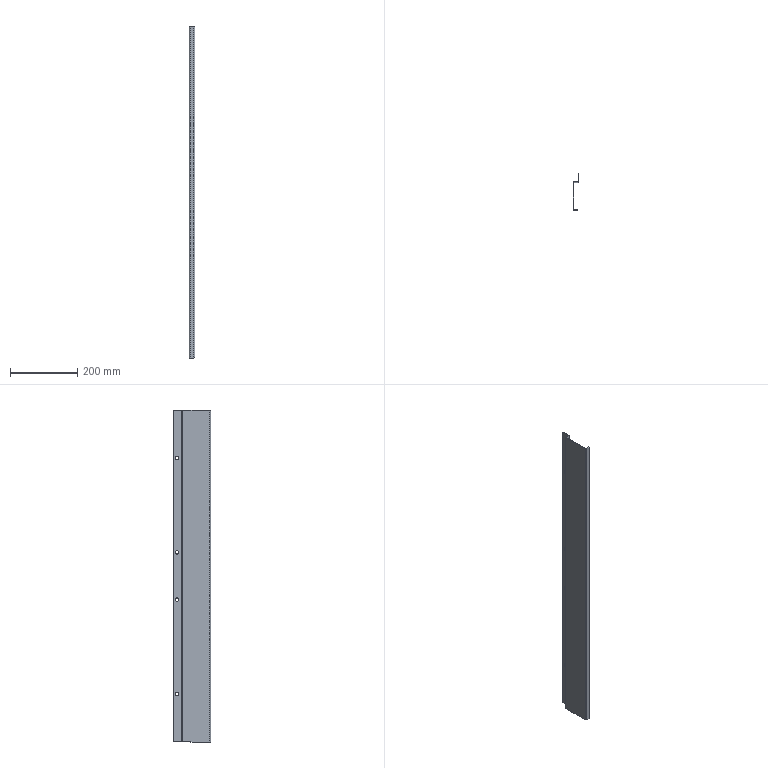Part | STEP file | 750038331 | 1 solid | 30 faces | box 16.25 x 110 x 985 mm | volume 264288 mm3 | plane 16 | cylinder 14 | commonest cylinder face diameters 10.5 x8 0.5 x3 4.5 x3
STEP:
#1=CARTESIAN_POINT('',(16.25,100.,355.25));
#2=VERTEX_POINT('',#1);
#3=CARTESIAN_POINT('',(16.25,100.,344.75));
#4=VERTEX_POINT('',#3);
#5=CARTESIAN_POINT('',(16.25,100.,350.));
#6=DIRECTION('',(1.,0.,0.));
#7=DIRECTION('',(0.,0.,1.));
#8=AXIS2_PLACEMENT_3D('',#5,#6,#7);
#9=CIRCLE('',#8,5.25);
#10=EDGE_CURVE('',#2,#4,#9,.T.);
#11=ORIENTED_EDGE('',*,*,#10,.T.);
#12=CARTESIAN_POINT('',(14.25,100.,344.75));
#13=VERTEX_POINT('',#12);
#14=CARTESIAN_POINT('',(1005.506,100.,344.75));
#15=DIRECTION('',(-1.,0.,0.));
#16=VECTOR('',#15,1000.);
#17=LINE('',#14,#16);
#18=EDGE_CURVE('',#4,#13,#17,.T.);
#19=ORIENTED_EDGE('',*,*,#18,.T.);
#20=CARTESIAN_POINT('',(14.25,100.,355.25));
#21=VERTEX_POINT('',#20);
#22=CARTESIAN_POINT('',(14.25,100.,350.));
#23=DIRECTION('',(1.,0.,0.));
#24=DIRECTION('',(0.,0.,1.));
#25=AXIS2_PLACEMENT_3D('',#22,#23,#24);
#26=CIRCLE('',#25,5.25);
#27=EDGE_CURVE('',#21,#13,#26,.T.);
#28=ORIENTED_EDGE('',*,*,#27,.F.);
#29=CARTESIAN_POINT('',(1005.506,100.,355.25));
#30=DIRECTION('',(-1.,0.,0.));
#31=VECTOR('',#30,1000.);
#32=LINE('',#29,#31);
#33=EDGE_CURVE('',#2,#21,#32,.T.);
#34=ORIENTED_EDGE('',*,*,#33,.F.);
#35=EDGE_LOOP('',(#11,#19,#28,#34));
#36=FACE_OUTER_BOUND('',#35,.T.);
#37=CARTESIAN_POINT('',(1005.506,100.,350.));
#38=DIRECTION('',(-1.,0.,0.));
#39=DIRECTION('',(0.,0.,1.));
#40=AXIS2_PLACEMENT_3D('',#37,#38,#39);
#41=CYLINDRICAL_SURFACE('',#40,5.25);
#42=ADVANCED_FACE('',(#36),#41,.F.);
#43=CARTESIAN_POINT('',(16.25,100.,75.25));
#44=VERTEX_POINT('',#43);
#45=CARTESIAN_POINT('',(16.25,100.,64.75));
#46=VERTEX_POINT('',#45);
#47=CARTESIAN_POINT('',(16.25,100.,70.));
#48=DIRECTION('',(1.,0.,0.));
#49=DIRECTION('',(0.,0.,1.));
#50=AXIS2_PLACEMENT_3D('',#47,#48,#49);
#51=CIRCLE('',#50,5.25);
#52=EDGE_CURVE('',#44,#46,#51,.T.);
#53=ORIENTED_EDGE('',*,*,#52,.T.);
#54=CARTESIAN_POINT('',(14.25,100.,64.75));
#55=VERTEX_POINT('',#54);
#56=CARTESIAN_POINT('',(1005.506,100.,64.75));
#57=DIRECTION('',(-1.,0.,0.));
#58=VECTOR('',#57,1000.);
#59=LINE('',#56,#58);
#60=EDGE_CURVE('',#46,#55,#59,.T.);
#61=ORIENTED_EDGE('',*,*,#60,.T.);
#62=CARTESIAN_POINT('',(14.25,100.,75.25));
#63=VERTEX_POINT('',#62);
#64=CARTESIAN_POINT('',(14.25,100.,70.));
#65=DIRECTION('',(1.,0.,0.));
#66=DIRECTION('',(0.,0.,1.));
#67=AXIS2_PLACEMENT_3D('',#64,#65,#66);
#68=CIRCLE('',#67,5.25);
#69=EDGE_CURVE('',#63,#55,#68,.T.);
#70=ORIENTED_EDGE('',*,*,#69,.F.);
#71=CARTESIAN_POINT('',(1005.506,100.,75.25));
#72=DIRECTION('',(-1.,0.,0.));
#73=VECTOR('',#72,1000.);
#74=LINE('',#71,#73);
#75=EDGE_CURVE('',#44,#63,#74,.T.);
#76=ORIENTED_EDGE('',*,*,#75,.F.);
#77=EDGE_LOOP('',(#53,#61,#70,#76));
#78=FACE_OUTER_BOUND('',#77,.T.);
#79=CARTESIAN_POINT('',(1005.506,100.,70.));
#80=DIRECTION('',(-1.,0.,0.));
#81=DIRECTION('',(0.,0.,1.));
#82=AXIS2_PLACEMENT_3D('',#79,#80,#81);
#83=CYLINDRICAL_SURFACE('',#82,5.25);
#84=ADVANCED_FACE('',(#78),#83,.F.);
#85=CARTESIAN_POINT('',(16.25,100.,-344.75));
#86=VERTEX_POINT('',#85);
#87=CARTESIAN_POINT('',(16.25,100.,-355.25));
#88=VERTEX_POINT('',#87);
#89=CARTESIAN_POINT('',(16.25,100.,-350.));
#90=DIRECTION('',(1.,0.,0.));
#91=DIRECTION('',(0.,0.,1.));
#92=AXIS2_PLACEMENT_3D('',#89,#90,#91);
#93=CIRCLE('',#92,5.25);
#94=EDGE_CURVE('',#86,#88,#93,.T.);
#95=ORIENTED_EDGE('',*,*,#94,.T.);
#96=CARTESIAN_POINT('',(14.25,100.,-355.25));
#97=VERTEX_POINT('',#96);
#98=CARTESIAN_POINT('',(1005.506,100.,-355.25));
#99=DIRECTION('',(-1.,0.,0.));
#100=VECTOR('',#99,1000.);
#101=LINE('',#98,#100);
#102=EDGE_CURVE('',#88,#97,#101,.T.);
#103=ORIENTED_EDGE('',*,*,#102,.T.);
#104=CARTESIAN_POINT('',(14.25,100.,-344.75));
#105=VERTEX_POINT('',#104);
#106=CARTESIAN_POINT('',(14.25,100.,-350.));
#107=DIRECTION('',(1.,0.,0.));
#108=DIRECTION('',(0.,0.,1.));
#109=AXIS2_PLACEMENT_3D('',#106,#107,#108);
#110=CIRCLE('',#109,5.25);
#111=EDGE_CURVE('',#105,#97,#110,.T.);
#112=ORIENTED_EDGE('',*,*,#111,.F.);
#113=CARTESIAN_POINT('',(1005.506,100.,-344.75));
#114=DIRECTION('',(-1.,0.,0.));
#115=VECTOR('',#114,1000.);
#116=LINE('',#113,#115);
#117=EDGE_CURVE('',#86,#105,#116,.T.);
#118=ORIENTED_EDGE('',*,*,#117,.F.);
#119=EDGE_LOOP('',(#95,#103,#112,#118));
#120=FACE_OUTER_BOUND('',#119,.T.);
#121=CARTESIAN_POINT('',(1005.506,100.,-350.));
#122=DIRECTION('',(-1.,0.,0.));
#123=DIRECTION('',(0.,0.,1.));
#124=AXIS2_PLACEMENT_3D('',#121,#122,#123);
#125=CYLINDRICAL_SURFACE('',#124,5.25);
#126=ADVANCED_FACE('',(#120),#125,.F.);
#127=CARTESIAN_POINT('',(16.25,100.,-64.75));
#128=VERTEX_POINT('',#127);
#129=CARTESIAN_POINT('',(16.25,100.,-75.25));
#130=VERTEX_POINT('',#129);
#131=CARTESIAN_POINT('',(16.25,100.,-70.));
#132=DIRECTION('',(1.,0.,0.));
#133=DIRECTION('',(0.,0.,1.));
#134=AXIS2_PLACEMENT_3D('',#131,#132,#133);
#135=CIRCLE('',#134,5.25);
#136=EDGE_CURVE('',#128,#130,#135,.T.);
#137=ORIENTED_EDGE('',*,*,#136,.T.);
#138=CARTESIAN_POINT('',(14.25,100.,-75.25));
#139=VERTEX_POINT('',#138);
#140=CARTESIAN_POINT('',(1005.506,100.,-75.25));
#141=DIRECTION('',(-1.,0.,0.));
#142=VECTOR('',#141,1000.);
#143=LINE('',#140,#142);
#144=EDGE_CURVE('',#130,#139,#143,.T.);
#145=ORIENTED_EDGE('',*,*,#144,.T.);
#146=CARTESIAN_POINT('',(14.25,100.,-64.75));
#147=VERTEX_POINT('',#146);
#148=CARTESIAN_POINT('',(14.25,100.,-70.));
#149=DIRECTION('',(1.,0.,0.));
#150=DIRECTION('',(0.,0.,1.));
#151=AXIS2_PLACEMENT_3D('',#148,#149,#150);
#152=CIRCLE('',#151,5.25);
#153=EDGE_CURVE('',#147,#139,#152,.T.);
#154=ORIENTED_EDGE('',*,*,#153,.F.);
#155=CARTESIAN_POINT('',(1005.506,100.,-64.75));
#156=DIRECTION('',(-1.,0.,0.));
#157=VECTOR('',#156,1000.);
#158=LINE('',#155,#157);
#159=EDGE_CURVE('',#128,#147,#158,.T.);
#160=ORIENTED_EDGE('',*,*,#159,.F.);
#161=EDGE_LOOP('',(#137,#145,#154,#160));
#162=FACE_OUTER_BOUND('',#161,.T.);
#163=CARTESIAN_POINT('',(1005.506,100.,-70.));
#164=DIRECTION('',(-1.,0.,0.));
#165=DIRECTION('',(0.,0.,1.));
#166=AXIS2_PLACEMENT_3D('',#163,#164,#165);
#167=CYLINDRICAL_SURFACE('',#166,5.25);
#168=ADVANCED_FACE('',(#162),#167,.F.);
#169=CARTESIAN_POINT('',(0.,83.75,491.5));
#170=VERTEX_POINT('',#169);
#171=CARTESIAN_POINT('',(0.,83.75,-491.5));
#172=VERTEX_POINT('',#171);
#173=CARTESIAN_POINT('',(0.,83.75,492.5));
#174=DIRECTION('',(0.,0.,-1.));
#175=VECTOR('',#174,1000.);
#176=LINE('',#173,#175);
#177=EDGE_CURVE('',#170,#172,#176,.T.);
#178=ORIENTED_EDGE('',*,*,#177,.T.);
#179=CARTESIAN_POINT('',(0.,58.,-491.5));
#180=VERTEX_POINT('',#179);
#181=CARTESIAN_POINT('',(0.,0.,-491.5));
#182=DIRECTION('',(0.,-1.,0.));
#183=VECTOR('',#182,1000.);
#184=LINE('',#181,#183);
#185=EDGE_CURVE('',#172,#180,#184,.T.);
#186=ORIENTED_EDGE('',*,*,#185,.T.);
#187=CARTESIAN_POINT('',(0.,58.,-492.5));
#188=VERTEX_POINT('',#187);
#189=CARTESIAN_POINT('',(0.,58.,492.5));
#190=DIRECTION('',(0.,0.,-1.));
#191=VECTOR('',#190,1000.);
#192=LINE('',#189,#191);
#193=EDGE_CURVE('',#180,#188,#192,.T.);
#194=ORIENTED_EDGE('',*,*,#193,.T.);
#195=CARTESIAN_POINT('',(0.,2.25,-492.5));
#196=VERTEX_POINT('',#195);
#197=CARTESIAN_POINT('',(0.,0.,-492.5));
#198=DIRECTION('',(0.,-1.,0.));
#199=VECTOR('',#198,1000.);
#200=LINE('',#197,#199);
#201=EDGE_CURVE('',#188,#196,#200,.T.);
#202=ORIENTED_EDGE('',*,*,#201,.T.);
#203=CARTESIAN_POINT('',(0.,2.25,492.5));
#204=VERTEX_POINT('',#203);
#205=CARTESIAN_POINT('',(0.,2.25,492.5));
#206=DIRECTION('',(0.,0.,1.));
#207=VECTOR('',#206,1000.);
#208=LINE('',#205,#207);
#209=EDGE_CURVE('',#196,#204,#208,.T.);
#210=ORIENTED_EDGE('',*,*,#209,.T.);
#211=CARTESIAN_POINT('',(0.,58.,492.5));
#212=VERTEX_POINT('',#211);
#213=CARTESIAN_POINT('',(0.,0.,492.5));
#214=DIRECTION('',(0.,1.,0.));
#215=VECTOR('',#214,1000.);
#216=LINE('',#213,#215);
#217=EDGE_CURVE('',#204,#212,#216,.T.);
#218=ORIENTED_EDGE('',*,*,#217,.T.);
#219=CARTESIAN_POINT('',(0.,58.,491.5));
#220=VERTEX_POINT('',#219);
#221=CARTESIAN_POINT('',(0.,58.,492.5));
#222=DIRECTION('',(0.,0.,1.));
#223=VECTOR('',#222,1000.);
#224=LINE('',#221,#223);
#225=EDGE_CURVE('',#220,#212,#224,.T.);
#226=ORIENTED_EDGE('',*,*,#225,.F.);
#227=CARTESIAN_POINT('',(0.,0.,491.5));
#228=DIRECTION('',(0.,1.,0.));
#229=VECTOR('',#228,1000.);
#230=LINE('',#227,#229);
#231=EDGE_CURVE('',#220,#170,#230,.T.);
#232=ORIENTED_EDGE('',*,*,#231,.T.);
#233=EDGE_LOOP('',(#178,#186,#194,#202,#210,#218,#226,#232));
#234=FACE_OUTER_BOUND('',#233,.T.);
#235=CARTESIAN_POINT('',(0.,0.,492.5));
#236=DIRECTION('',(-1.,0.,0.));
#237=DIRECTION('',(0.,0.,1.));
#238=AXIS2_PLACEMENT_3D('',#235,#236,#237);
#239=PLANE('',#238);
#240=ADVANCED_FACE('',(#234),#239,.T.);
#241=CARTESIAN_POINT('',(2.25,86.,-491.5));
#242=VERTEX_POINT('',#241);
#243=CARTESIAN_POINT('',(2.25,83.75,-491.5));
#244=DIRECTION('',(0.,0.,-1.));
#245=DIRECTION('',(-1.,0.,0.));
#246=AXIS2_PLACEMENT_3D('',#243,#244,#245);
#247=CIRCLE('',#246,2.25);
#248=EDGE_CURVE('',#172,#242,#247,.T.);
#249=ORIENTED_EDGE('',*,*,#248,.T.);
#250=CARTESIAN_POINT('',(14.,86.,-491.5));
#251=VERTEX_POINT('',#250);
#252=CARTESIAN_POINT('',(14.,86.,-491.5));
#253=DIRECTION('',(1.,0.,0.));
#254=VECTOR('',#253,1000.);
#255=LINE('',#252,#254);
#256=EDGE_CURVE('',#242,#251,#255,.T.);
#257=ORIENTED_EDGE('',*,*,#256,.T.);
#258=CARTESIAN_POINT('',(14.25,86.25,-491.5));
#259=VERTEX_POINT('',#258);
#260=CARTESIAN_POINT('',(14.,86.25,-491.5));
#261=DIRECTION('',(0.,0.,1.));
#262=DIRECTION('',(-1.,0.,0.));
#263=AXIS2_PLACEMENT_3D('',#260,#261,#262);
#264=CIRCLE('',#263,0.25);
#265=EDGE_CURVE('',#251,#259,#264,.T.);
#266=ORIENTED_EDGE('',*,*,#265,.T.);
#267=CARTESIAN_POINT('',(14.25,110.,-491.5));
#268=VERTEX_POINT('',#267);
#269=CARTESIAN_POINT('',(14.25,86.25,-491.5));
#270=DIRECTION('',(0.,1.,0.));
#271=VECTOR('',#270,1000.);
#272=LINE('',#269,#271);
#273=EDGE_CURVE('',#259,#268,#272,.T.);
#274=ORIENTED_EDGE('',*,*,#273,.T.);
#275=CARTESIAN_POINT('',(16.25,110.,-491.5));
#276=VERTEX_POINT('',#275);
#277=CARTESIAN_POINT('',(14.,110.,-491.5));
#278=DIRECTION('',(1.,0.,0.));
#279=VECTOR('',#278,1000.);
#280=LINE('',#277,#279);
#281=EDGE_CURVE('',#268,#276,#280,.T.);
#282=ORIENTED_EDGE('',*,*,#281,.T.);
#283=CARTESIAN_POINT('',(16.25,86.25,-491.5));
#284=VERTEX_POINT('',#283);
#285=CARTESIAN_POINT('',(16.25,86.25,-491.5));
#286=DIRECTION('',(0.,-1.,0.));
#287=VECTOR('',#286,1000.);
#288=LINE('',#285,#287);
#289=EDGE_CURVE('',#276,#284,#288,.T.);
#290=ORIENTED_EDGE('',*,*,#289,.T.);
#291=CARTESIAN_POINT('',(14.,84.,-491.5));
#292=VERTEX_POINT('',#291);
#293=CARTESIAN_POINT('',(14.,86.25,-491.5));
#294=DIRECTION('',(0.,0.,-1.));
#295=DIRECTION('',(-1.,0.,0.));
#296=AXIS2_PLACEMENT_3D('',#293,#294,#295);
#297=CIRCLE('',#296,2.25);
#298=EDGE_CURVE('',#284,#292,#297,.T.);
#299=ORIENTED_EDGE('',*,*,#298,.T.);
#300=CARTESIAN_POINT('',(2.25,84.,-491.5));
#301=VERTEX_POINT('',#300);
#302=CARTESIAN_POINT('',(14.,84.,-491.5));
#303=DIRECTION('',(-1.,0.,0.));
#304=VECTOR('',#303,1000.);
#305=LINE('',#302,#304);
#306=EDGE_CURVE('',#292,#301,#305,.T.);
#307=ORIENTED_EDGE('',*,*,#306,.T.);
#308=CARTESIAN_POINT('',(2.,83.75,-491.5));
#309=VERTEX_POINT('',#308);
#310=CARTESIAN_POINT('',(2.25,83.75,-491.5));
#311=DIRECTION('',(0.,0.,1.));
#312=DIRECTION('',(-1.,0.,0.));
#313=AXIS2_PLACEMENT_3D('',#310,#311,#312);
#314=CIRCLE('',#313,0.25);
#315=EDGE_CURVE('',#301,#309,#314,.T.);
#316=ORIENTED_EDGE('',*,*,#315,.T.);
#317=CARTESIAN_POINT('',(2.,58.,-491.5));
#318=VERTEX_POINT('',#317);
#319=CARTESIAN_POINT('',(2.,86.25,-491.5));
#320=DIRECTION('',(0.,-1.,0.));
#321=VECTOR('',#320,1000.);
#322=LINE('',#319,#321);
#323=EDGE_CURVE('',#309,#318,#322,.T.);
#324=ORIENTED_EDGE('',*,*,#323,.T.);
#325=CARTESIAN_POINT('',(14.,58.,-491.5));
#326=DIRECTION('',(-1.,0.,0.));
#327=VECTOR('',#326,1000.);
#328=LINE('',#325,#327);
#329=EDGE_CURVE('',#318,#180,#328,.T.);
#330=ORIENTED_EDGE('',*,*,#329,.T.);
#331=ORIENTED_EDGE('',*,*,#185,.F.);
#332=EDGE_LOOP('',(#249,#257,#266,#274,#282,#290,#299,#307,#316,#324,#330,#331));
#333=FACE_OUTER_BOUND('',#332,.T.);
#334=CARTESIAN_POINT('',(14.,86.25,-491.5));
#335=DIRECTION('',(0.,0.,-1.));
#336=DIRECTION('',(-1.,0.,0.));
#337=AXIS2_PLACEMENT_3D('',#334,#335,#336);
#338=PLANE('',#337);
#339=ADVANCED_FACE('',(#333),#338,.T.);
#340=CARTESIAN_POINT('',(2.25,86.,491.5));
#341=VERTEX_POINT('',#340);
#342=CARTESIAN_POINT('',(2.25,83.75,491.5));
#343=DIRECTION('',(0.,0.,-1.));
#344=DIRECTION('',(-1.,0.,0.));
#345=AXIS2_PLACEMENT_3D('',#342,#343,#344);
#346=CIRCLE('',#345,2.25);
#347=EDGE_CURVE('',#170,#341,#346,.T.);
#348=ORIENTED_EDGE('',*,*,#347,.T.);
#349=CARTESIAN_POINT('',(2.25,86.,492.5));
#350=DIRECTION('',(0.,0.,-1.));
#351=VECTOR('',#350,1000.);
#352=LINE('',#349,#351);
#353=EDGE_CURVE('',#341,#242,#352,.T.);
#354=ORIENTED_EDGE('',*,*,#353,.T.);
#355=ORIENTED_EDGE('',*,*,#248,.F.);
#356=ORIENTED_EDGE('',*,*,#177,.F.);
#357=EDGE_LOOP('',(#348,#354,#355,#356));
#358=FACE_OUTER_BOUND('',#357,.T.);
#359=CARTESIAN_POINT('',(2.25,83.75,492.5));
#360=DIRECTION('',(0.,0.,-1.));
#361=DIRECTION('',(-1.,0.,0.));
#362=AXIS2_PLACEMENT_3D('',#359,#360,#361);
#363=CYLINDRICAL_SURFACE('',#362,2.25);
#364=ADVANCED_FACE('',(#358),#363,.T.);
#365=CARTESIAN_POINT('',(16.25,86.25,491.5));
#366=VERTEX_POINT('',#365);
#367=CARTESIAN_POINT('',(16.25,110.,491.5));
#368=VERTEX_POINT('',#367);
#369=CARTESIAN_POINT('',(16.25,86.25,491.5));
#370=DIRECTION('',(0.,1.,0.));
#371=VECTOR('',#370,1000.);
#372=LINE('',#369,#371);
#373=EDGE_CURVE('',#366,#368,#372,.T.);
#374=ORIENTED_EDGE('',*,*,#373,.T.);
#375=CARTESIAN_POINT('',(14.25,110.,491.5));
#376=VERTEX_POINT('',#375);
#377=CARTESIAN_POINT('',(14.25,110.,491.5));
#378=DIRECTION('',(-1.,0.,0.));
#379=VECTOR('',#378,1000.);
#380=LINE('',#377,#379);
#381=EDGE_CURVE('',#368,#376,#380,.T.);
#382=ORIENTED_EDGE('',*,*,#381,.T.);
#383=CARTESIAN_POINT('',(14.25,86.25,491.5));
#384=VERTEX_POINT('',#383);
#385=CARTESIAN_POINT('',(14.25,86.25,491.5));
#386=DIRECTION('',(0.,-1.,0.));
#387=VECTOR('',#386,1000.);
#388=LINE('',#385,#387);
#389=EDGE_CURVE('',#376,#384,#388,.T.);
#390=ORIENTED_EDGE('',*,*,#389,.T.);
#391=CARTESIAN_POINT('',(14.,86.,491.5));
#392=VERTEX_POINT('',#391);
#393=CARTESIAN_POINT('',(14.,86.25,491.5));
#394=DIRECTION('',(0.,0.,-1.));
#395=DIRECTION('',(-1.,0.,0.));
#396=AXIS2_PLACEMENT_3D('',#393,#394,#395);
#397=CIRCLE('',#396,0.25);
#398=EDGE_CURVE('',#384,#392,#397,.T.);
#399=ORIENTED_EDGE('',*,*,#398,.T.);
#400=CARTESIAN_POINT('',(14.25,86.,491.5));
#401=DIRECTION('',(-1.,0.,0.));
#402=VECTOR('',#401,1000.);
#403=LINE('',#400,#402);
#404=EDGE_CURVE('',#392,#341,#403,.T.);
#405=ORIENTED_EDGE('',*,*,#404,.T.);
#406=ORIENTED_EDGE('',*,*,#347,.F.);
#407=ORIENTED_EDGE('',*,*,#231,.F.);
#408=CARTESIAN_POINT('',(2.,58.,491.5));
#409=VERTEX_POINT('',#408);
#410=CARTESIAN_POINT('',(14.25,58.,491.5));
#411=DIRECTION('',(1.,0.,0.));
#412=VECTOR('',#411,1000.);
#413=LINE('',#410,#412);
#414=EDGE_CURVE('',#220,#409,#413,.T.);
#415=ORIENTED_EDGE('',*,*,#414,.T.);
#416=CARTESIAN_POINT('',(2.,83.75,491.5));
#417=VERTEX_POINT('',#416);
#418=CARTESIAN_POINT('',(2.,86.25,491.5));
#419=DIRECTION('',(0.,1.,0.));
#420=VECTOR('',#419,1000.);
#421=LINE('',#418,#420);
#422=EDGE_CURVE('',#409,#417,#421,.T.);
#423=ORIENTED_EDGE('',*,*,#422,.T.);
#424=CARTESIAN_POINT('',(2.25,84.,491.5));
#425=VERTEX_POINT('',#424);
#426=CARTESIAN_POINT('',(2.25,83.75,491.5));
#427=DIRECTION('',(0.,0.,-1.));
#428=DIRECTION('',(-1.,0.,0.));
#429=AXIS2_PLACEMENT_3D('',#426,#427,#428);
#430=CIRCLE('',#429,0.25);
#431=EDGE_CURVE('',#417,#425,#430,.T.);
#432=ORIENTED_EDGE('',*,*,#431,.T.);
#433=CARTESIAN_POINT('',(14.,84.,491.5));
#434=VERTEX_POINT('',#433);
#435=CARTESIAN_POINT('',(14.25,84.,491.5));
#436=DIRECTION('',(1.,0.,0.));
#437=VECTOR('',#436,1000.);
#438=LINE('',#435,#437);
#439=EDGE_CURVE('',#425,#434,#438,.T.);
#440=ORIENTED_EDGE('',*,*,#439,.T.);
#441=CARTESIAN_POINT('',(14.,86.25,491.5));
#442=DIRECTION('',(0.,0.,1.));
#443=DIRECTION('',(-1.,0.,0.));
#444=AXIS2_PLACEMENT_3D('',#441,#442,#443);
#445=CIRCLE('',#444,2.25);
#446=EDGE_CURVE('',#434,#366,#445,.T.);
#447=ORIENTED_EDGE('',*,*,#446,.T.);
#448=EDGE_LOOP('',(#374,#382,#390,#399,#405,#406,#407,#415,#423,#432,#440,#447));
#449=FACE_OUTER_BOUND('',#448,.T.);
#450=CARTESIAN_POINT('',(14.25,86.25,491.5));
#451=DIRECTION('',(0.,0.,1.));
#452=DIRECTION('',(1.,0.,0.));
#453=AXIS2_PLACEMENT_3D('',#450,#451,#452);
#454=PLANE('',#453);
#455=ADVANCED_FACE('',(#449),#454,.T.);
#456=CARTESIAN_POINT('',(14.,2.,492.5));
#457=VERTEX_POINT('',#456);
#458=CARTESIAN_POINT('',(2.25,2.,492.5));
#459=VERTEX_POINT('',#458);
#460=CARTESIAN_POINT('',(0.,2.,492.5));
#461=DIRECTION('',(-1.,0.,0.));
#462=VECTOR('',#461,1000.);
#463=LINE('',#460,#462);
#464=EDGE_CURVE('',#457,#459,#463,.T.);
#465=ORIENTED_EDGE('',*,*,#464,.T.);
#466=CARTESIAN_POINT('',(2.,2.25,492.5));
#467=VERTEX_POINT('',#466);
#468=CARTESIAN_POINT('',(2.25,2.25,492.5));
#469=DIRECTION('',(0.,0.,-1.));
#470=DIRECTION('',(-1.,0.,0.));
#471=AXIS2_PLACEMENT_3D('',#468,#469,#470);
#472=CIRCLE('',#471,0.25);
#473=EDGE_CURVE('',#459,#467,#472,.T.);
#474=ORIENTED_EDGE('',*,*,#473,.T.);
#475=CARTESIAN_POINT('',(2.,58.,492.5));
#476=VERTEX_POINT('',#475);
#477=CARTESIAN_POINT('',(2.,86.,492.5));
#478=DIRECTION('',(0.,1.,0.));
#479=VECTOR('',#478,1000.);
#480=LINE('',#477,#479);
#481=EDGE_CURVE('',#467,#476,#480,.T.);
#482=ORIENTED_EDGE('',*,*,#481,.T.);
#483=CARTESIAN_POINT('',(0.,58.,492.5));
#484=DIRECTION('',(-1.,0.,0.));
#485=VECTOR('',#484,1000.);
#486=LINE('',#483,#485);
#487=EDGE_CURVE('',#476,#212,#486,.T.);
#488=ORIENTED_EDGE('',*,*,#487,.T.);
#489=ORIENTED_EDGE('',*,*,#217,.F.);
#490=CARTESIAN_POINT('',(2.25,0.,492.5));
#491=VERTEX_POINT('',#490);
#492=CARTESIAN_POINT('',(2.25,2.25,492.5));
#493=DIRECTION('',(0.,0.,1.));
#494=DIRECTION('',(-1.,0.,0.));
#495=AXIS2_PLACEMENT_3D('',#492,#493,#494);
#496=CIRCLE('',#495,2.25);
#497=EDGE_CURVE('',#204,#491,#496,.T.);
#498=ORIENTED_EDGE('',*,*,#497,.T.);
#499=CARTESIAN_POINT('',(14.,0.,492.5));
#500=VERTEX_POINT('',#499);
#501=CARTESIAN_POINT('',(0.,0.,492.5));
#502=DIRECTION('',(1.,0.,0.));
#503=VECTOR('',#502,1000.);
#504=LINE('',#501,#503);
#505=EDGE_CURVE('',#491,#500,#504,.T.);
#506=ORIENTED_EDGE('',*,*,#505,.T.);
#507=CARTESIAN_POINT('',(14.,86.,492.5));
#508=DIRECTION('',(0.,1.,0.));
#509=VECTOR('',#508,1000.);
#510=LINE('',#507,#509);
#511=EDGE_CURVE('',#500,#457,#510,.T.);
#512=ORIENTED_EDGE('',*,*,#511,.T.);
#513=EDGE_LOOP('',(#465,#474,#482,#488,#489,#498,#506,#512));
#514=FACE_OUTER_BOUND('',#513,.T.);
#515=CARTESIAN_POINT('',(0.,86.,492.5));
#516=DIRECTION('',(0.,0.,1.));
#517=DIRECTION('',(1.,0.,0.));
#518=AXIS2_PLACEMENT_3D('',#515,#516,#517);
#519=PLANE('',#518);
#520=ADVANCED_FACE('',(#514),#519,.T.);
#521=ORIENTED_EDGE('',*,*,#497,.F.);
#522=ORIENTED_EDGE('',*,*,#209,.F.);
#523=CARTESIAN_POINT('',(2.25,0.,-492.5));
#524=VERTEX_POINT('',#523);
#525=CARTESIAN_POINT('',(2.25,2.25,-492.5));
#526=DIRECTION('',(0.,0.,1.));
#527=DIRECTION('',(-1.,0.,0.));
#528=AXIS2_PLACEMENT_3D('',#525,#526,#527);
#529=CIRCLE('',#528,2.25);
#530=EDGE_CURVE('',#196,#524,#529,.T.);
#531=ORIENTED_EDGE('',*,*,#530,.T.);
#532=CARTESIAN_POINT('',(2.25,0.,492.5));
#533=DIRECTION('',(0.,0.,1.));
#534=VECTOR('',#533,1000.);
#535=LINE('',#532,#534);
#536=EDGE_CURVE('',#524,#491,#535,.T.);
#537=ORIENTED_EDGE('',*,*,#536,.T.);
#538=EDGE_LOOP('',(#521,#522,#531,#537));
#539=FACE_OUTER_BOUND('',#538,.T.);
#540=CARTESIAN_POINT('',(2.25,2.25,492.5));
#541=DIRECTION('',(0.,0.,-1.));
#542=DIRECTION('',(-1.,0.,0.));
#543=AXIS2_PLACEMENT_3D('',#540,#541,#542);
#544=CYLINDRICAL_SURFACE('',#543,2.25);
#545=ADVANCED_FACE('',(#539),#544,.T.);
#546=CARTESIAN_POINT('',(2.,2.25,-492.5));
#547=VERTEX_POINT('',#546);
#548=CARTESIAN_POINT('',(2.,58.,-492.5));
#549=VERTEX_POINT('',#548);
#550=CARTESIAN_POINT('',(2.,0.,-492.5));
#551=DIRECTION('',(0.,1.,0.));
#552=VECTOR('',#551,1000.);
#553=LINE('',#550,#552);
#554=EDGE_CURVE('',#547,#549,#553,.T.);
#555=ORIENTED_EDGE('',*,*,#554,.F.);
#556=CARTESIAN_POINT('',(2.25,2.,-492.5));
#557=VERTEX_POINT('',#556);
#558=CARTESIAN_POINT('',(2.25,2.25,-492.5));
#559=DIRECTION('',(0.,0.,1.));
#560=DIRECTION('',(-1.,0.,0.));
#561=AXIS2_PLACEMENT_3D('',#558,#559,#560);
#562=CIRCLE('',#561,0.25);
#563=EDGE_CURVE('',#547,#557,#562,.T.);
#564=ORIENTED_EDGE('',*,*,#563,.T.);
#565=CARTESIAN_POINT('',(14.,2.,-492.5));
#566=VERTEX_POINT('',#565);
#567=CARTESIAN_POINT('',(14.,2.,-492.5));
#568=DIRECTION('',(-1.,0.,0.));
#569=VECTOR('',#568,1000.);
#570=LINE('',#567,#569);
#571=EDGE_CURVE('',#566,#557,#570,.T.);
#572=ORIENTED_EDGE('',*,*,#571,.F.);
#573=CARTESIAN_POINT('',(14.,0.,-492.5));
#574=VERTEX_POINT('',#573);
#575=CARTESIAN_POINT('',(14.,0.,-492.5));
#576=DIRECTION('',(0.,1.,0.));
#577=VECTOR('',#576,1000.);
#578=LINE('',#575,#577);
#579=EDGE_CURVE('',#574,#566,#578,.T.);
#580=ORIENTED_EDGE('',*,*,#579,.F.);
#581=CARTESIAN_POINT('',(14.,0.,-492.5));
#582=DIRECTION('',(1.,0.,0.));
#583=VECTOR('',#582,1000.);
#584=LINE('',#581,#583);
#585=EDGE_CURVE('',#524,#574,#584,.T.);
#586=ORIENTED_EDGE('',*,*,#585,.F.);
#587=ORIENTED_EDGE('',*,*,#530,.F.);
#588=ORIENTED_EDGE('',*,*,#201,.F.);
#589=CARTESIAN_POINT('',(14.,58.,-492.5));
#590=DIRECTION('',(-1.,0.,0.));
#591=VECTOR('',#590,1000.);
#592=LINE('',#589,#591);
#593=EDGE_CURVE('',#549,#188,#592,.T.);
#594=ORIENTED_EDGE('',*,*,#593,.F.);
#595=EDGE_LOOP('',(#555,#564,#572,#580,#586,#587,#588,#594));
#596=FACE_OUTER_BOUND('',#595,.T.);
#597=CARTESIAN_POINT('',(14.,0.,-492.5));
#598=DIRECTION('',(0.,0.,1.));
#599=DIRECTION('',(1.,0.,0.));
#600=AXIS2_PLACEMENT_3D('',#597,#598,#599);
#601=PLANE('',#600);
#602=ADVANCED_FACE('',(#596),#601,.F.);
#603=ORIENTED_EDGE('',*,*,#404,.F.);
#604=CARTESIAN_POINT('',(14.,86.,492.5));
#605=DIRECTION('',(0.,0.,-1.));
#606=VECTOR('',#605,1000.);
#607=LINE('',#604,#606);
#608=EDGE_CURVE('',#392,#251,#607,.T.);
#609=ORIENTED_EDGE('',*,*,#608,.T.);
#610=ORIENTED_EDGE('',*,*,#256,.F.);
#611=ORIENTED_EDGE('',*,*,#353,.F.);
#612=EDGE_LOOP('',(#603,#609,#610,#611));
#613=FACE_OUTER_BOUND('',#612,.T.);
#614=CARTESIAN_POINT('',(0.,86.,492.5));
#615=DIRECTION('',(0.,1.,0.));
#616=DIRECTION('',(0.,0.,1.));
#617=AXIS2_PLACEMENT_3D('',#614,#615,#616);
#618=PLANE('',#617);
#619=ADVANCED_FACE('',(#613),#618,.T.);
#620=ORIENTED_EDGE('',*,*,#193,.F.);
#621=ORIENTED_EDGE('',*,*,#329,.F.);
#622=CARTESIAN_POINT('',(2.,58.,492.5));
#623=DIRECTION('',(0.,0.,1.));
#624=VECTOR('',#623,1000.);
#625=LINE('',#622,#624);
#626=EDGE_CURVE('',#549,#318,#625,.T.);
#627=ORIENTED_EDGE('',*,*,#626,.F.);
#628=ORIENTED_EDGE('',*,*,#593,.T.);
#629=EDGE_LOOP('',(#620,#621,#627,#628));
#630=FACE_OUTER_BOUND('',#629,.T.);
#631=CARTESIAN_POINT('',(0.,58.,492.5));
#632=DIRECTION('',(0.,-1.,0.));
#633=DIRECTION('',(0.,0.,-1.));
#634=AXIS2_PLACEMENT_3D('',#631,#632,#633);
#635=PLANE('',#634);
#636=ADVANCED_FACE('',(#630),#635,.F.);
#637=ORIENTED_EDGE('',*,*,#323,.F.);
#638=CARTESIAN_POINT('',(2.,83.75,492.5));
#639=DIRECTION('',(0.,0.,-1.));
#640=VECTOR('',#639,1000.);
#641=LINE('',#638,#640);
#642=EDGE_CURVE('',#417,#309,#641,.T.);
#643=ORIENTED_EDGE('',*,*,#642,.F.);
#644=ORIENTED_EDGE('',*,*,#422,.F.);
#645=CARTESIAN_POINT('',(2.,58.,492.5));
#646=DIRECTION('',(0.,0.,-1.));
#647=VECTOR('',#646,1000.);
#648=LINE('',#645,#647);
#649=EDGE_CURVE('',#476,#409,#648,.T.);
#650=ORIENTED_EDGE('',*,*,#649,.F.);
#651=ORIENTED_EDGE('',*,*,#481,.F.);
#652=CARTESIAN_POINT('',(2.,2.25,492.5));
#653=DIRECTION('',(0.,0.,1.));
#654=VECTOR('',#653,1000.);
#655=LINE('',#652,#654);
#656=EDGE_CURVE('',#547,#467,#655,.T.);
#657=ORIENTED_EDGE('',*,*,#656,.F.);
#658=ORIENTED_EDGE('',*,*,#554,.T.);
#659=ORIENTED_EDGE('',*,*,#626,.T.);
#660=EDGE_LOOP('',(#637,#643,#644,#650,#651,#657,#658,#659));
#661=FACE_OUTER_BOUND('',#660,.T.);
#662=CARTESIAN_POINT('',(2.,0.,492.5));
#663=DIRECTION('',(-1.,0.,0.));
#664=DIRECTION('',(0.,0.,1.));
#665=AXIS2_PLACEMENT_3D('',#662,#663,#664);
#666=PLANE('',#665);
#667=ADVANCED_FACE('',(#661),#666,.F.);
#668=ORIENTED_EDGE('',*,*,#306,.F.);
#669=CARTESIAN_POINT('',(14.,84.,492.5));
#670=DIRECTION('',(0.,0.,-1.));
#671=VECTOR('',#670,1000.);
#672=LINE('',#669,#671);
#673=EDGE_CURVE('',#434,#292,#672,.T.);
#674=ORIENTED_EDGE('',*,*,#673,.F.);
#675=ORIENTED_EDGE('',*,*,#439,.F.);
#676=CARTESIAN_POINT('',(2.25,84.,492.5));
#677=DIRECTION('',(0.,0.,1.));
#678=VECTOR('',#677,1000.);
#679=LINE('',#676,#678);
#680=EDGE_CURVE('',#301,#425,#679,.T.);
#681=ORIENTED_EDGE('',*,*,#680,.F.);
#682=EDGE_LOOP('',(#668,#674,#675,#681));
#683=FACE_OUTER_BOUND('',#682,.T.);
#684=CARTESIAN_POINT('',(0.,84.,492.5));
#685=DIRECTION('',(0.,1.,0.));
#686=DIRECTION('',(0.,0.,1.));
#687=AXIS2_PLACEMENT_3D('',#684,#685,#686);
#688=PLANE('',#687);
#689=ADVANCED_FACE('',(#683),#688,.F.);
#690=ORIENTED_EDGE('',*,*,#446,.F.);
#691=ORIENTED_EDGE('',*,*,#673,.T.);
#692=ORIENTED_EDGE('',*,*,#298,.F.);
#693=CARTESIAN_POINT('',(16.25,86.25,491.5));
#694=DIRECTION('',(0.,0.,1.));
#695=VECTOR('',#694,1000.);
#696=LINE('',#693,#695);
#697=EDGE_CURVE('',#284,#366,#696,.T.);
#698=ORIENTED_EDGE('',*,*,#697,.T.);
#699=EDGE_LOOP('',(#690,#691,#692,#698));
#700=FACE_OUTER_BOUND('',#699,.T.);
#701=CARTESIAN_POINT('',(14.,86.25,491.5));
#702=DIRECTION('',(0.,0.,-1.));
#703=DIRECTION('',(-1.,0.,0.));
#704=AXIS2_PLACEMENT_3D('',#701,#702,#703);
#705=CYLINDRICAL_SURFACE('',#704,2.25);
#706=ADVANCED_FACE('',(#700),#705,.T.);
#707=CARTESIAN_POINT('',(16.25,110.,491.5));
#708=DIRECTION('',(0.,0.,-1.));
#709=VECTOR('',#708,1000.);
#710=LINE('',#707,#709);
#711=EDGE_CURVE('',#368,#276,#710,.T.);
#712=ORIENTED_EDGE('',*,*,#711,.F.);
#713=ORIENTED_EDGE('',*,*,#373,.F.);
#714=ORIENTED_EDGE('',*,*,#697,.F.);
#715=ORIENTED_EDGE('',*,*,#289,.F.);
#716=EDGE_LOOP('',(#712,#713,#714,#715));
#717=FACE_OUTER_BOUND('',#716,.T.);
#718=ORIENTED_EDGE('',*,*,#10,.F.);
#719=CARTESIAN_POINT('',(16.25,100.,350.));
#720=DIRECTION('',(1.,0.,0.));
#721=DIRECTION('',(0.,0.,1.));
#722=AXIS2_PLACEMENT_3D('',#719,#720,#721);
#723=CIRCLE('',#722,5.25);
#724=EDGE_CURVE('',#4,#2,#723,.T.);
#725=ORIENTED_EDGE('',*,*,#724,.F.);
#726=EDGE_LOOP('',(#718,#725));
#727=FACE_BOUND('',#726,.T.);
#728=ORIENTED_EDGE('',*,*,#52,.F.);
#729=CARTESIAN_POINT('',(16.25,100.,70.));
#730=DIRECTION('',(1.,0.,0.));
#731=DIRECTION('',(0.,0.,1.));
#732=AXIS2_PLACEMENT_3D('',#729,#730,#731);
#733=CIRCLE('',#732,5.25);
#734=EDGE_CURVE('',#46,#44,#733,.T.);
#735=ORIENTED_EDGE('',*,*,#734,.F.);
#736=EDGE_LOOP('',(#728,#735));
#737=FACE_BOUND('',#736,.T.);
#738=ORIENTED_EDGE('',*,*,#94,.F.);
#739=CARTESIAN_POINT('',(16.25,100.,-350.));
#740=DIRECTION('',(1.,0.,0.));
#741=DIRECTION('',(0.,0.,1.));
#742=AXIS2_PLACEMENT_3D('',#739,#740,#741);
#743=CIRCLE('',#742,5.25);
#744=EDGE_CURVE('',#88,#86,#743,.T.);
#745=ORIENTED_EDGE('',*,*,#744,.F.);
#746=EDGE_LOOP('',(#738,#745));
#747=FACE_BOUND('',#746,.T.);
#748=ORIENTED_EDGE('',*,*,#136,.F.);
#749=CARTESIAN_POINT('',(16.25,100.,-70.));
#750=DIRECTION('',(1.,0.,0.));
#751=DIRECTION('',(0.,0.,1.));
#752=AXIS2_PLACEMENT_3D('',#749,#750,#751);
#753=CIRCLE('',#752,5.25);
#754=EDGE_CURVE('',#130,#128,#753,.T.);
#755=ORIENTED_EDGE('',*,*,#754,.F.);
#756=EDGE_LOOP('',(#748,#755));
#757=FACE_BOUND('',#756,.T.);
#758=CARTESIAN_POINT('',(16.25,86.25,491.5));
#759=DIRECTION('',(-1.,0.,0.));
#760=DIRECTION('',(0.,0.,1.));
#761=AXIS2_PLACEMENT_3D('',#758,#759,#760);
#762=PLANE('',#761);
#763=ADVANCED_FACE('',(#717,#727,#737,#747,#757),#762,.F.);
#764=ORIENTED_EDGE('',*,*,#281,.F.);
#765=CARTESIAN_POINT('',(14.25,110.,491.5));
#766=DIRECTION('',(0.,0.,1.));
#767=VECTOR('',#766,1000.);
#768=LINE('',#765,#767);
#769=EDGE_CURVE('',#268,#376,#768,.T.);
#770=ORIENTED_EDGE('',*,*,#769,.T.);
#771=ORIENTED_EDGE('',*,*,#381,.F.);
#772=ORIENTED_EDGE('',*,*,#711,.T.);
#773=EDGE_LOOP('',(#764,#770,#771,#772));
#774=FACE_OUTER_BOUND('',#773,.T.);
#775=CARTESIAN_POINT('',(14.25,110.,491.5));
#776=DIRECTION('',(0.,1.,0.));
#777=DIRECTION('',(0.,0.,1.));
#778=AXIS2_PLACEMENT_3D('',#775,#776,#777);
#779=PLANE('',#778);
#780=ADVANCED_FACE('',(#774),#779,.T.);
#781=ORIENTED_EDGE('',*,*,#389,.F.);
#782=ORIENTED_EDGE('',*,*,#769,.F.);
#783=ORIENTED_EDGE('',*,*,#273,.F.);
#784=CARTESIAN_POINT('',(14.25,86.25,491.5));
#785=DIRECTION('',(0.,0.,1.));
#786=VECTOR('',#785,1000.);
#787=LINE('',#784,#786);
#788=EDGE_CURVE('',#259,#384,#787,.T.);
#789=ORIENTED_EDGE('',*,*,#788,.T.);
#790=EDGE_LOOP('',(#781,#782,#783,#789));
#791=FACE_OUTER_BOUND('',#790,.T.);
#792=ORIENTED_EDGE('',*,*,#27,.T.);
#793=CARTESIAN_POINT('',(14.25,100.,350.));
#794=DIRECTION('',(1.,0.,0.));
#795=DIRECTION('',(0.,0.,1.));
#796=AXIS2_PLACEMENT_3D('',#793,#794,#795);
#797=CIRCLE('',#796,5.25);
#798=EDGE_CURVE('',#13,#21,#797,.T.);
#799=ORIENTED_EDGE('',*,*,#798,.T.);
#800=EDGE_LOOP('',(#792,#799));
#801=FACE_BOUND('',#800,.T.);
#802=ORIENTED_EDGE('',*,*,#69,.T.);
#803=CARTESIAN_POINT('',(14.25,100.,70.));
#804=DIRECTION('',(1.,0.,0.));
#805=DIRECTION('',(0.,0.,1.));
#806=AXIS2_PLACEMENT_3D('',#803,#804,#805);
#807=CIRCLE('',#806,5.25);
#808=EDGE_CURVE('',#55,#63,#807,.T.);
#809=ORIENTED_EDGE('',*,*,#808,.T.);
#810=EDGE_LOOP('',(#802,#809));
#811=FACE_BOUND('',#810,.T.);
#812=ORIENTED_EDGE('',*,*,#111,.T.);
#813=CARTESIAN_POINT('',(14.25,100.,-350.));
#814=DIRECTION('',(1.,0.,0.));
#815=DIRECTION('',(0.,0.,1.));
#816=AXIS2_PLACEMENT_3D('',#813,#814,#815);
#817=CIRCLE('',#816,5.25);
#818=EDGE_CURVE('',#97,#105,#817,.T.);
#819=ORIENTED_EDGE('',*,*,#818,.T.);
#820=EDGE_LOOP('',(#812,#819));
#821=FACE_BOUND('',#820,.T.);
#822=ORIENTED_EDGE('',*,*,#153,.T.);
#823=CARTESIAN_POINT('',(14.25,100.,-70.));
#824=DIRECTION('',(1.,0.,0.));
#825=DIRECTION('',(0.,0.,1.));
#826=AXIS2_PLACEMENT_3D('',#823,#824,#825);
#827=CIRCLE('',#826,5.25);
#828=EDGE_CURVE('',#139,#147,#827,.T.);
#829=ORIENTED_EDGE('',*,*,#828,.T.);
#830=EDGE_LOOP('',(#822,#829));
#831=FACE_BOUND('',#830,.T.);
#832=CARTESIAN_POINT('',(14.25,86.25,491.5));
#833=DIRECTION('',(-1.,0.,0.));
#834=DIRECTION('',(0.,0.,1.));
#835=AXIS2_PLACEMENT_3D('',#832,#833,#834);
#836=PLANE('',#835);
#837=ADVANCED_FACE('',(#791,#801,#811,#821,#831),#836,.T.);
#838=ORIENTED_EDGE('',*,*,#487,.F.);
#839=ORIENTED_EDGE('',*,*,#649,.T.);
#840=ORIENTED_EDGE('',*,*,#414,.F.);
#841=ORIENTED_EDGE('',*,*,#225,.T.);
#842=EDGE_LOOP('',(#838,#839,#840,#841));
#843=FACE_OUTER_BOUND('',#842,.T.);
#844=CARTESIAN_POINT('',(0.,58.,492.5));
#845=DIRECTION('',(0.,1.,0.));
#846=DIRECTION('',(0.,0.,1.));
#847=AXIS2_PLACEMENT_3D('',#844,#845,#846);
#848=PLANE('',#847);
#849=ADVANCED_FACE('',(#843),#848,.T.);
#850=CARTESIAN_POINT('',(2.25,2.,492.5));
#851=DIRECTION('',(0.,0.,-1.));
#852=VECTOR('',#851,1000.);
#853=LINE('',#850,#852);
#854=EDGE_CURVE('',#459,#557,#853,.T.);
#855=ORIENTED_EDGE('',*,*,#854,.F.);
#856=ORIENTED_EDGE('',*,*,#464,.F.);
#857=CARTESIAN_POINT('',(14.,2.,492.5));
#858=DIRECTION('',(0.,0.,1.));
#859=VECTOR('',#858,1000.);
#860=LINE('',#857,#859);
#861=EDGE_CURVE('',#566,#457,#860,.T.);
#862=ORIENTED_EDGE('',*,*,#861,.F.);
#863=ORIENTED_EDGE('',*,*,#571,.T.);
#864=EDGE_LOOP('',(#855,#856,#862,#863));
#865=FACE_OUTER_BOUND('',#864,.T.);
#866=CARTESIAN_POINT('',(14.,2.,492.5));
#867=DIRECTION('',(0.,-1.,0.));
#868=DIRECTION('',(0.,0.,-1.));
#869=AXIS2_PLACEMENT_3D('',#866,#867,#868);
#870=PLANE('',#869);
#871=ADVANCED_FACE('',(#865),#870,.F.);
#872=ORIENTED_EDGE('',*,*,#511,.F.);
#873=CARTESIAN_POINT('',(14.,0.,492.5));
#874=DIRECTION('',(0.,0.,1.));
#875=VECTOR('',#874,1000.);
#876=LINE('',#873,#875);
#877=EDGE_CURVE('',#574,#500,#876,.T.);
#878=ORIENTED_EDGE('',*,*,#877,.F.);
#879=ORIENTED_EDGE('',*,*,#579,.T.);
#880=ORIENTED_EDGE('',*,*,#861,.T.);
#881=EDGE_LOOP('',(#872,#878,#879,#880));
#882=FACE_OUTER_BOUND('',#881,.T.);
#883=CARTESIAN_POINT('',(14.,0.,492.5));
#884=DIRECTION('',(-1.,0.,0.));
#885=DIRECTION('',(0.,0.,1.));
#886=AXIS2_PLACEMENT_3D('',#883,#884,#885);
#887=PLANE('',#886);
#888=ADVANCED_FACE('',(#882),#887,.F.);
#889=ORIENTED_EDGE('',*,*,#505,.F.);
#890=ORIENTED_EDGE('',*,*,#536,.F.);
#891=ORIENTED_EDGE('',*,*,#585,.T.);
#892=ORIENTED_EDGE('',*,*,#877,.T.);
#893=EDGE_LOOP('',(#889,#890,#891,#892));
#894=FACE_OUTER_BOUND('',#893,.T.);
#895=CARTESIAN_POINT('',(14.,0.,492.5));
#896=DIRECTION('',(0.,-1.,0.));
#897=DIRECTION('',(0.,0.,-1.));
#898=AXIS2_PLACEMENT_3D('',#895,#896,#897);
#899=PLANE('',#898);
#900=ADVANCED_FACE('',(#894),#899,.T.);
#901=ORIENTED_EDGE('',*,*,#608,.F.);
#902=ORIENTED_EDGE('',*,*,#398,.F.);
#903=ORIENTED_EDGE('',*,*,#788,.F.);
#904=ORIENTED_EDGE('',*,*,#265,.F.);
#905=EDGE_LOOP('',(#901,#902,#903,#904));
#906=FACE_OUTER_BOUND('',#905,.T.);
#907=CARTESIAN_POINT('',(14.,86.25,491.5));
#908=DIRECTION('',(0.,0.,-1.));
#909=DIRECTION('',(-1.,0.,0.));
#910=AXIS2_PLACEMENT_3D('',#907,#908,#909);
#911=CYLINDRICAL_SURFACE('',#910,0.25);
#912=ADVANCED_FACE('',(#906),#911,.F.);
#913=ORIENTED_EDGE('',*,*,#315,.F.);
#914=ORIENTED_EDGE('',*,*,#680,.T.);
#915=ORIENTED_EDGE('',*,*,#431,.F.);
#916=ORIENTED_EDGE('',*,*,#642,.T.);
#917=EDGE_LOOP('',(#913,#914,#915,#916));
#918=FACE_OUTER_BOUND('',#917,.T.);
#919=CARTESIAN_POINT('',(2.25,83.75,492.5));
#920=DIRECTION('',(0.,0.,-1.));
#921=DIRECTION('',(-1.,0.,0.));
#922=AXIS2_PLACEMENT_3D('',#919,#920,#921);
#923=CYLINDRICAL_SURFACE('',#922,0.25);
#924=ADVANCED_FACE('',(#918),#923,.F.);
#925=ORIENTED_EDGE('',*,*,#656,.T.);
#926=ORIENTED_EDGE('',*,*,#473,.F.);
#927=ORIENTED_EDGE('',*,*,#854,.T.);
#928=ORIENTED_EDGE('',*,*,#563,.F.);
#929=EDGE_LOOP('',(#925,#926,#927,#928));
#930=FACE_OUTER_BOUND('',#929,.T.);
#931=CARTESIAN_POINT('',(2.25,2.25,492.5));
#932=DIRECTION('',(0.,0.,-1.));
#933=DIRECTION('',(-1.,0.,0.));
#934=AXIS2_PLACEMENT_3D('',#931,#932,#933);
#935=CYLINDRICAL_SURFACE('',#934,0.25);
#936=ADVANCED_FACE('',(#930),#935,.F.);
#937=ORIENTED_EDGE('',*,*,#18,.F.);
#938=ORIENTED_EDGE('',*,*,#724,.T.);
#939=ORIENTED_EDGE('',*,*,#33,.T.);
#940=ORIENTED_EDGE('',*,*,#798,.F.);
#941=EDGE_LOOP('',(#937,#938,#939,#940));
#942=FACE_OUTER_BOUND('',#941,.T.);
#943=CARTESIAN_POINT('',(1005.506,100.,350.));
#944=DIRECTION('',(-1.,0.,0.));
#945=DIRECTION('',(0.,0.,1.));
#946=AXIS2_PLACEMENT_3D('',#943,#944,#945);
#947=CYLINDRICAL_SURFACE('',#946,5.25);
#948=ADVANCED_FACE('',(#942),#947,.F.);
#949=ORIENTED_EDGE('',*,*,#60,.F.);
#950=ORIENTED_EDGE('',*,*,#734,.T.);
#951=ORIENTED_EDGE('',*,*,#75,.T.);
#952=ORIENTED_EDGE('',*,*,#808,.F.);
#953=EDGE_LOOP('',(#949,#950,#951,#952));
#954=FACE_OUTER_BOUND('',#953,.T.);
#955=CARTESIAN_POINT('',(1005.506,100.,70.));
#956=DIRECTION('',(-1.,0.,0.));
#957=DIRECTION('',(0.,0.,1.));
#958=AXIS2_PLACEMENT_3D('',#955,#956,#957);
#959=CYLINDRICAL_SURFACE('',#958,5.25);
#960=ADVANCED_FACE('',(#954),#959,.F.);
#961=ORIENTED_EDGE('',*,*,#102,.F.);
#962=ORIENTED_EDGE('',*,*,#744,.T.);
#963=ORIENTED_EDGE('',*,*,#117,.T.);
#964=ORIENTED_EDGE('',*,*,#818,.F.);
#965=EDGE_LOOP('',(#961,#962,#963,#964));
#966=FACE_OUTER_BOUND('',#965,.T.);
#967=CARTESIAN_POINT('',(1005.506,100.,-350.));
#968=DIRECTION('',(-1.,0.,0.));
#969=DIRECTION('',(0.,0.,1.));
#970=AXIS2_PLACEMENT_3D('',#967,#968,#969);
#971=CYLINDRICAL_SURFACE('',#970,5.25);
#972=ADVANCED_FACE('',(#966),#971,.F.);
#973=ORIENTED_EDGE('',*,*,#144,.F.);
#974=ORIENTED_EDGE('',*,*,#754,.T.);
#975=ORIENTED_EDGE('',*,*,#159,.T.);
#976=ORIENTED_EDGE('',*,*,#828,.F.);
#977=EDGE_LOOP('',(#973,#974,#975,#976));
#978=FACE_OUTER_BOUND('',#977,.T.);
#979=CARTESIAN_POINT('',(1005.506,100.,-70.));
#980=DIRECTION('',(-1.,0.,0.));
#981=DIRECTION('',(0.,0.,1.));
#982=AXIS2_PLACEMENT_3D('',#979,#980,#981);
#983=CYLINDRICAL_SURFACE('',#982,5.25);
#984=ADVANCED_FACE('',(#978),#983,.F.);
#985=CLOSED_SHELL('',(#42,#84,#126,#168,#240,#339,#364,#455,#520,#545,#602,#619,#636,#667,#689,#706,#763,#780,#837,#849,#871,#888,#900,#912,#924,#936,#948,#960,#972,#984));
#986=MANIFOLD_SOLID_BREP('',#985);
#987=CARTESIAN_POINT('',(0.,0.,0.));
#988=DIRECTION('',(0.,0.,1.));
#989=DIRECTION('',(1.,0.,0.));
#990=AXIS2_PLACEMENT_3D('',#987,#988,#989);
#991=(LENGTH_UNIT()NAMED_UNIT(*)SI_UNIT(.MILLI.,.METRE.));
#992=UNCERTAINTY_MEASURE_WITH_UNIT(LENGTH_MEASURE(0.00001),#991,'','');
#993=(NAMED_UNIT(*)PLANE_ANGLE_UNIT()SI_UNIT($,.RADIAN.));
#994=(NAMED_UNIT(*)SI_UNIT($,.STERADIAN.)SOLID_ANGLE_UNIT());
#995=(GEOMETRIC_REPRESENTATION_CONTEXT(3)GLOBAL_UNCERTAINTY_ASSIGNED_CONTEXT((#992))GLOBAL_UNIT_ASSIGNED_CONTEXT((#991,#993,#994))REPRESENTATION_CONTEXT('',''));
#996=ADVANCED_BREP_SHAPE_REPRESENTATION('',(#986,#990),#995);